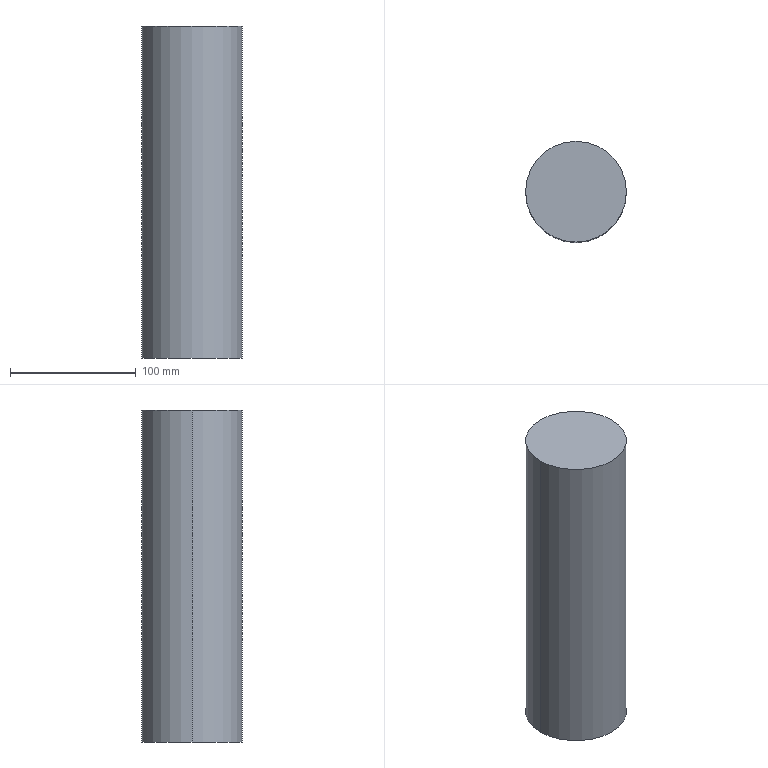Part | SolidWorks | features Extrusion 1 | 1 solid | 4 faces | box 80 x 80 x 263.5 mm | volume 1324495 mm3 | cylinder 2 | plane 2 | commonest cylinder face diameters 80 x2
STEP:
#1=CARTESIAN_POINT('',(40.,0.,263.5));
#2=VERTEX_POINT('',#1);
#3=CARTESIAN_POINT('',(-40.,0.,263.5));
#4=VERTEX_POINT('',#3);
#5=CARTESIAN_POINT('',(0.,0.,263.5));
#6=DIRECTION('',(0.,0.,1.));
#7=DIRECTION('',(1.,0.,0.));
#8=AXIS2_PLACEMENT_3D('',#5,#6,#7);
#9=CIRCLE('',#8,40.);
#10=EDGE_CURVE('',#2,#4,#9,.T.);
#11=ORIENTED_EDGE('',*,*,#10,.F.);
#12=CARTESIAN_POINT('',(40.,0.,0.));
#13=VERTEX_POINT('',#12);
#14=CARTESIAN_POINT('',(40.,0.,263.5));
#15=DIRECTION('',(0.,0.,-1.));
#16=VECTOR('',#15,1000.);
#17=LINE('',#14,#16);
#18=EDGE_CURVE('',#2,#13,#17,.T.);
#19=ORIENTED_EDGE('',*,*,#18,.T.);
#20=CARTESIAN_POINT('',(-40.,0.,0.));
#21=VERTEX_POINT('',#20);
#22=CARTESIAN_POINT('',(0.,0.,0.));
#23=DIRECTION('',(0.,0.,1.));
#24=DIRECTION('',(1.,0.,0.));
#25=AXIS2_PLACEMENT_3D('',#22,#23,#24);
#26=CIRCLE('',#25,40.);
#27=EDGE_CURVE('',#13,#21,#26,.T.);
#28=ORIENTED_EDGE('',*,*,#27,.T.);
#29=CARTESIAN_POINT('',(-40.,0.,263.5));
#30=DIRECTION('',(0.,0.,-1.));
#31=VECTOR('',#30,1000.);
#32=LINE('',#29,#31);
#33=EDGE_CURVE('',#4,#21,#32,.T.);
#34=ORIENTED_EDGE('',*,*,#33,.F.);
#35=EDGE_LOOP('',(#11,#19,#28,#34));
#36=FACE_OUTER_BOUND('',#35,.T.);
#37=CARTESIAN_POINT('',(0.,0.,263.5));
#38=DIRECTION('',(0.,0.,-1.));
#39=DIRECTION('',(-1.,0.,0.));
#40=AXIS2_PLACEMENT_3D('',#37,#38,#39);
#41=CYLINDRICAL_SURFACE('',#40,40.);
#42=ADVANCED_FACE('',(#36),#41,.T.);
#43=ORIENTED_EDGE('',*,*,#18,.F.);
#44=CARTESIAN_POINT('',(0.,0.,263.5));
#45=DIRECTION('',(0.,0.,1.));
#46=DIRECTION('',(1.,0.,0.));
#47=AXIS2_PLACEMENT_3D('',#44,#45,#46);
#48=CIRCLE('',#47,40.);
#49=EDGE_CURVE('',#4,#2,#48,.T.);
#50=ORIENTED_EDGE('',*,*,#49,.F.);
#51=ORIENTED_EDGE('',*,*,#33,.T.);
#52=CARTESIAN_POINT('',(0.,0.,0.));
#53=DIRECTION('',(0.,0.,1.));
#54=DIRECTION('',(1.,0.,0.));
#55=AXIS2_PLACEMENT_3D('',#52,#53,#54);
#56=CIRCLE('',#55,40.);
#57=EDGE_CURVE('',#21,#13,#56,.T.);
#58=ORIENTED_EDGE('',*,*,#57,.T.);
#59=EDGE_LOOP('',(#43,#50,#51,#58));
#60=FACE_OUTER_BOUND('',#59,.T.);
#61=CARTESIAN_POINT('',(0.,0.,263.5));
#62=DIRECTION('',(0.,0.,-1.));
#63=DIRECTION('',(-1.,0.,0.));
#64=AXIS2_PLACEMENT_3D('',#61,#62,#63);
#65=CYLINDRICAL_SURFACE('',#64,40.);
#66=ADVANCED_FACE('',(#60),#65,.T.);
#67=ORIENTED_EDGE('',*,*,#49,.T.);
#68=ORIENTED_EDGE('',*,*,#10,.T.);
#69=EDGE_LOOP('',(#67,#68));
#70=FACE_OUTER_BOUND('',#69,.T.);
#71=CARTESIAN_POINT('',(0.,0.,263.5));
#72=DIRECTION('',(0.,0.,1.));
#73=DIRECTION('',(1.,0.,0.));
#74=AXIS2_PLACEMENT_3D('',#71,#72,#73);
#75=PLANE('',#74);
#76=ADVANCED_FACE('',(#70),#75,.T.);
#77=ORIENTED_EDGE('',*,*,#57,.F.);
#78=ORIENTED_EDGE('',*,*,#27,.F.);
#79=EDGE_LOOP('',(#77,#78));
#80=FACE_OUTER_BOUND('',#79,.T.);
#81=CARTESIAN_POINT('',(0.,0.,0.));
#82=DIRECTION('',(0.,0.,1.));
#83=DIRECTION('',(1.,0.,0.));
#84=AXIS2_PLACEMENT_3D('',#81,#82,#83);
#85=PLANE('',#84);
#86=ADVANCED_FACE('',(#80),#85,.F.);
#87=CLOSED_SHELL('',(#42,#66,#76,#86));
#88=MANIFOLD_SOLID_BREP('',#87);
#89=CARTESIAN_POINT('',(0.,0.,0.));
#90=DIRECTION('',(0.,0.,1.));
#91=DIRECTION('',(1.,0.,0.));
#92=AXIS2_PLACEMENT_3D('',#89,#90,#91);
#93=(LENGTH_UNIT()NAMED_UNIT(*)SI_UNIT(.MILLI.,.METRE.));
#94=UNCERTAINTY_MEASURE_WITH_UNIT(LENGTH_MEASURE(0.00001),#93,'','');
#95=(NAMED_UNIT(*)PLANE_ANGLE_UNIT()SI_UNIT($,.RADIAN.));
#96=(NAMED_UNIT(*)SI_UNIT($,.STERADIAN.)SOLID_ANGLE_UNIT());
#97=(GEOMETRIC_REPRESENTATION_CONTEXT(3)GLOBAL_UNCERTAINTY_ASSIGNED_CONTEXT((#94))GLOBAL_UNIT_ASSIGNED_CONTEXT((#93,#95,#96))REPRESENTATION_CONTEXT('',''));
#98=ADVANCED_BREP_SHAPE_REPRESENTATION('',(#88,#92),#97);